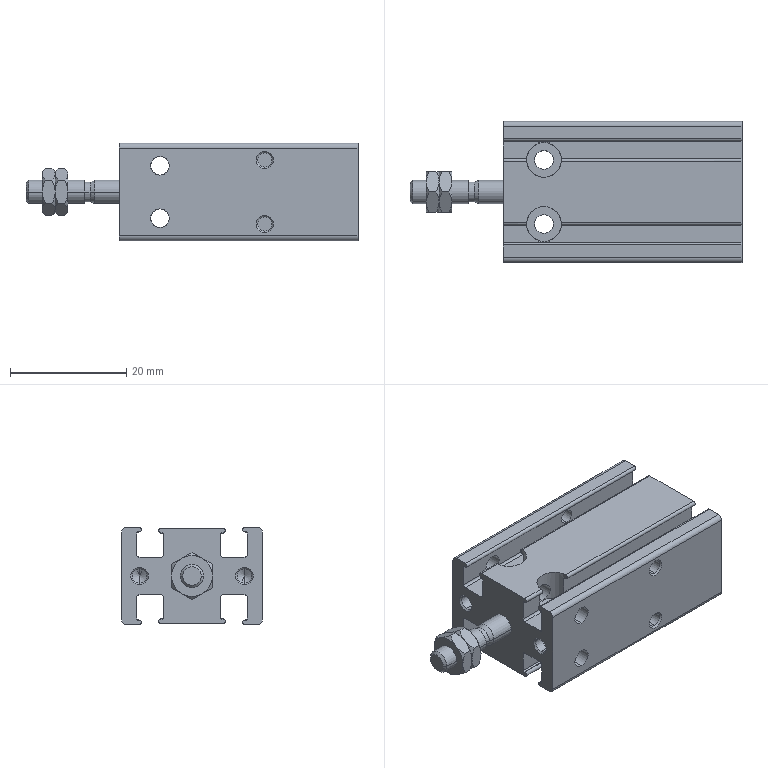Part | STEP file | 4 solids | 294 faces | box 57 x 24.2 x 16.7 mm | volume 11440 mm3 | cylinder 148 | cone 78 | plane 68 | commonest cylinder face diameters 0.8 x38 0.4 x18 2.459 x16 3.2 x16 6 x16 4 x6